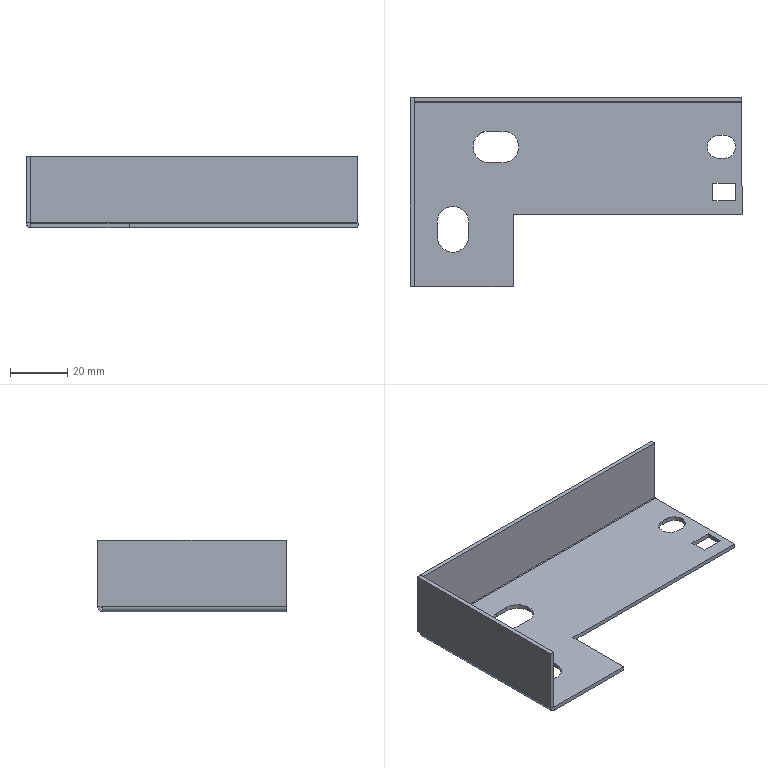Part | 1 solid | 43 faces | box 116 x 66 x 25 mm | volume 14104 mm3 | plane 31 | cylinder 12 | commonest cylinder face diameters 11 x5 8 x3 0.4 x2 3.4 x2
STEP:
#1=CARTESIAN_POINT('',(-20.,15.8,-1.5));
#2=VERTEX_POINT('',#1);
#3=CARTESIAN_POINT('',(-25.5,21.3,-1.5));
#4=VERTEX_POINT('',#3);
#5=CARTESIAN_POINT('',(-25.5,15.8,-1.5));
#6=DIRECTION('',(0.,0.,1.));
#7=DIRECTION('',(1.,0.,0.));
#8=AXIS2_PLACEMENT_3D('',#5,#6,#7);
#9=CIRCLE('',#8,5.5);
#10=EDGE_CURVE('',#2,#4,#9,.T.);
#11=ORIENTED_EDGE('',*,*,#10,.F.);
#12=CARTESIAN_POINT('',(-20.,15.8,0.));
#13=VERTEX_POINT('',#12);
#14=CARTESIAN_POINT('',(-20.,15.8,-10.));
#15=DIRECTION('',(0.,0.,1.));
#16=VECTOR('',#15,1000.);
#17=LINE('',#14,#16);
#18=EDGE_CURVE('',#2,#13,#17,.T.);
#19=ORIENTED_EDGE('',*,*,#18,.T.);
#20=CARTESIAN_POINT('',(-25.5,21.3,0.));
#21=VERTEX_POINT('',#20);
#22=CARTESIAN_POINT('',(-25.5,15.8,0.));
#23=DIRECTION('',(0.,0.,1.));
#24=DIRECTION('',(1.,0.,0.));
#25=AXIS2_PLACEMENT_3D('',#22,#23,#24);
#26=CIRCLE('',#25,5.5);
#27=EDGE_CURVE('',#13,#21,#26,.T.);
#28=ORIENTED_EDGE('',*,*,#27,.T.);
#29=CARTESIAN_POINT('',(-25.5,21.3,-10.));
#30=DIRECTION('',(0.,0.,1.));
#31=VECTOR('',#30,1000.);
#32=LINE('',#29,#31);
#33=EDGE_CURVE('',#4,#21,#32,.T.);
#34=ORIENTED_EDGE('',*,*,#33,.F.);
#35=EDGE_LOOP('',(#11,#19,#28,#34));
#36=FACE_OUTER_BOUND('',#35,.T.);
#37=CARTESIAN_POINT('',(-25.5,15.8,-10.));
#38=DIRECTION('',(0.,0.,1.));
#39=DIRECTION('',(1.,0.,0.));
#40=AXIS2_PLACEMENT_3D('',#37,#38,#39);
#41=CYLINDRICAL_SURFACE('',#40,5.5);
#42=ADVANCED_FACE('',(#36),#41,.F.);
#43=CARTESIAN_POINT('',(55.8,15.8,-1.5));
#44=VERTEX_POINT('',#43);
#45=CARTESIAN_POINT('',(51.8,19.8,-1.5));
#46=VERTEX_POINT('',#45);
#47=CARTESIAN_POINT('',(51.8,15.8,-1.5));
#48=DIRECTION('',(0.,0.,1.));
#49=DIRECTION('',(1.,0.,0.));
#50=AXIS2_PLACEMENT_3D('',#47,#48,#49);
#51=CIRCLE('',#50,4.);
#52=EDGE_CURVE('',#44,#46,#51,.T.);
#53=ORIENTED_EDGE('',*,*,#52,.F.);
#54=CARTESIAN_POINT('',(55.8,15.8,0.));
#55=VERTEX_POINT('',#54);
#56=CARTESIAN_POINT('',(55.8,15.8,-10.));
#57=DIRECTION('',(0.,0.,1.));
#58=VECTOR('',#57,1000.);
#59=LINE('',#56,#58);
#60=EDGE_CURVE('',#44,#55,#59,.T.);
#61=ORIENTED_EDGE('',*,*,#60,.T.);
#62=CARTESIAN_POINT('',(51.8,19.8,0.));
#63=VERTEX_POINT('',#62);
#64=CARTESIAN_POINT('',(51.8,15.8,0.));
#65=DIRECTION('',(0.,0.,1.));
#66=DIRECTION('',(1.,0.,0.));
#67=AXIS2_PLACEMENT_3D('',#64,#65,#66);
#68=CIRCLE('',#67,4.);
#69=EDGE_CURVE('',#55,#63,#68,.T.);
#70=ORIENTED_EDGE('',*,*,#69,.T.);
#71=CARTESIAN_POINT('',(51.8,19.8,-10.));
#72=DIRECTION('',(0.,0.,1.));
#73=VECTOR('',#72,1000.);
#74=LINE('',#71,#73);
#75=EDGE_CURVE('',#46,#63,#74,.T.);
#76=ORIENTED_EDGE('',*,*,#75,.F.);
#77=EDGE_LOOP('',(#53,#61,#70,#76));
#78=FACE_OUTER_BOUND('',#77,.T.);
#79=CARTESIAN_POINT('',(51.8,15.8,-10.));
#80=DIRECTION('',(0.,0.,1.));
#81=DIRECTION('',(1.,0.,0.));
#82=AXIS2_PLACEMENT_3D('',#79,#80,#81);
#83=CYLINDRICAL_SURFACE('',#82,4.);
#84=ADVANCED_FACE('',(#78),#83,.F.);
#85=CARTESIAN_POINT('',(-30.5,21.3,-1.5));
#86=VERTEX_POINT('',#85);
#87=CARTESIAN_POINT('',(0.,21.3,-1.5));
#88=DIRECTION('',(-1.,0.,0.));
#89=VECTOR('',#88,1000.);
#90=LINE('',#87,#89);
#91=EDGE_CURVE('',#4,#86,#90,.T.);
#92=ORIENTED_EDGE('',*,*,#91,.T.);
#93=CARTESIAN_POINT('',(-30.5,10.3,-1.5));
#94=VERTEX_POINT('',#93);
#95=CARTESIAN_POINT('',(-30.5,15.8,-1.5));
#96=DIRECTION('',(0.,0.,1.));
#97=DIRECTION('',(1.,0.,0.));
#98=AXIS2_PLACEMENT_3D('',#95,#96,#97);
#99=CIRCLE('',#98,5.5);
#100=EDGE_CURVE('',#86,#94,#99,.T.);
#101=ORIENTED_EDGE('',*,*,#100,.T.);
#102=CARTESIAN_POINT('',(-25.5,10.3,-1.5));
#103=VERTEX_POINT('',#102);
#104=CARTESIAN_POINT('',(0.,10.3,-1.5));
#105=DIRECTION('',(1.,0.,0.));
#106=VECTOR('',#105,1000.);
#107=LINE('',#104,#106);
#108=EDGE_CURVE('',#94,#103,#107,.T.);
#109=ORIENTED_EDGE('',*,*,#108,.T.);
#110=CARTESIAN_POINT('',(-25.5,15.8,-1.5));
#111=DIRECTION('',(0.,0.,1.));
#112=DIRECTION('',(1.,0.,0.));
#113=AXIS2_PLACEMENT_3D('',#110,#111,#112);
#114=CIRCLE('',#113,5.5);
#115=EDGE_CURVE('',#103,#2,#114,.T.);
#116=ORIENTED_EDGE('',*,*,#115,.T.);
#117=ORIENTED_EDGE('',*,*,#10,.T.);
#118=EDGE_LOOP('',(#92,#101,#109,#116,#117));
#119=FACE_BOUND('',#118,.T.);
#120=CARTESIAN_POINT('',(58.,-8.,-1.5));
#121=VERTEX_POINT('',#120);
#122=CARTESIAN_POINT('',(58.,31.3,-1.5));
#123=VERTEX_POINT('',#122);
#124=CARTESIAN_POINT('',(58.,33.,-1.5));
#125=DIRECTION('',(0.,1.,0.));
#126=VECTOR('',#125,1000.);
#127=LINE('',#124,#126);
#128=EDGE_CURVE('',#121,#123,#127,.T.);
#129=ORIENTED_EDGE('',*,*,#128,.F.);
#130=CARTESIAN_POINT('',(-22.,-8.,-1.5));
#131=VERTEX_POINT('',#130);
#132=CARTESIAN_POINT('',(0.,-8.,-1.5));
#133=DIRECTION('',(-1.,0.,0.));
#134=VECTOR('',#133,1000.);
#135=LINE('',#132,#134);
#136=EDGE_CURVE('',#121,#131,#135,.T.);
#137=ORIENTED_EDGE('',*,*,#136,.T.);
#138=CARTESIAN_POINT('',(-22.,-33.,-1.5));
#139=VERTEX_POINT('',#138);
#140=CARTESIAN_POINT('',(-22.,0.,-1.5));
#141=DIRECTION('',(0.,-1.,0.));
#142=VECTOR('',#141,1000.);
#143=LINE('',#140,#142);
#144=EDGE_CURVE('',#131,#139,#143,.T.);
#145=ORIENTED_EDGE('',*,*,#144,.T.);
#146=CARTESIAN_POINT('',(-56.3,-33.,-1.5));
#147=VERTEX_POINT('',#146);
#148=CARTESIAN_POINT('',(-58.,-33.,-1.5));
#149=DIRECTION('',(1.,0.,0.));
#150=VECTOR('',#149,1000.);
#151=LINE('',#148,#150);
#152=EDGE_CURVE('',#147,#139,#151,.T.);
#153=ORIENTED_EDGE('',*,*,#152,.F.);
#154=CARTESIAN_POINT('',(-56.3,31.3,-1.5));
#155=VERTEX_POINT('',#154);
#156=CARTESIAN_POINT('',(-56.3,-33.,-1.5));
#157=DIRECTION('',(0.,1.,0.));
#158=VECTOR('',#157,1000.);
#159=LINE('',#156,#158);
#160=EDGE_CURVE('',#147,#155,#159,.T.);
#161=ORIENTED_EDGE('',*,*,#160,.T.);
#162=CARTESIAN_POINT('',(-56.3,31.3,-1.5));
#163=DIRECTION('',(1.,0.,0.));
#164=VECTOR('',#163,1000.);
#165=LINE('',#162,#164);
#166=EDGE_CURVE('',#155,#123,#165,.T.);
#167=ORIENTED_EDGE('',*,*,#166,.T.);
#168=EDGE_LOOP('',(#129,#137,#145,#153,#161,#167));
#169=FACE_OUTER_BOUND('',#168,.T.);
#170=CARTESIAN_POINT('',(-37.5,-15.5,-1.5));
#171=VERTEX_POINT('',#170);
#172=CARTESIAN_POINT('',(-37.5,-10.5,-1.5));
#173=VERTEX_POINT('',#172);
#174=CARTESIAN_POINT('',(-37.5,0.,-1.5));
#175=DIRECTION('',(0.,1.,0.));
#176=VECTOR('',#175,1000.);
#177=LINE('',#174,#176);
#178=EDGE_CURVE('',#171,#173,#177,.T.);
#179=ORIENTED_EDGE('',*,*,#178,.T.);
#180=CARTESIAN_POINT('',(-48.5,-10.5,-1.5));
#181=VERTEX_POINT('',#180);
#182=CARTESIAN_POINT('',(-43.,-10.5,-1.5));
#183=DIRECTION('',(0.,0.,1.));
#184=DIRECTION('',(1.,0.,0.));
#185=AXIS2_PLACEMENT_3D('',#182,#183,#184);
#186=CIRCLE('',#185,5.5);
#187=EDGE_CURVE('',#173,#181,#186,.T.);
#188=ORIENTED_EDGE('',*,*,#187,.T.);
#189=CARTESIAN_POINT('',(-48.5,-15.5,-1.5));
#190=VERTEX_POINT('',#189);
#191=CARTESIAN_POINT('',(-48.5,0.,-1.5));
#192=DIRECTION('',(0.,-1.,0.));
#193=VECTOR('',#192,1000.);
#194=LINE('',#191,#193);
#195=EDGE_CURVE('',#181,#190,#194,.T.);
#196=ORIENTED_EDGE('',*,*,#195,.T.);
#197=CARTESIAN_POINT('',(-43.,-15.5,-1.5));
#198=DIRECTION('',(0.,0.,1.));
#199=DIRECTION('',(1.,0.,0.));
#200=AXIS2_PLACEMENT_3D('',#197,#198,#199);
#201=CIRCLE('',#200,5.5);
#202=EDGE_CURVE('',#190,#171,#201,.T.);
#203=ORIENTED_EDGE('',*,*,#202,.T.);
#204=EDGE_LOOP('',(#179,#188,#196,#203));
#205=FACE_BOUND('',#204,.T.);
#206=CARTESIAN_POINT('',(49.8,19.8,-1.5));
#207=VERTEX_POINT('',#206);
#208=CARTESIAN_POINT('',(0.,19.8,-1.5));
#209=DIRECTION('',(-1.,0.,0.));
#210=VECTOR('',#209,1000.);
#211=LINE('',#208,#210);
#212=EDGE_CURVE('',#46,#207,#211,.T.);
#213=ORIENTED_EDGE('',*,*,#212,.T.);
#214=CARTESIAN_POINT('',(49.8,11.8,-1.5));
#215=VERTEX_POINT('',#214);
#216=CARTESIAN_POINT('',(49.8,15.8,-1.5));
#217=DIRECTION('',(0.,0.,1.));
#218=DIRECTION('',(1.,0.,0.));
#219=AXIS2_PLACEMENT_3D('',#216,#217,#218);
#220=CIRCLE('',#219,4.);
#221=EDGE_CURVE('',#207,#215,#220,.T.);
#222=ORIENTED_EDGE('',*,*,#221,.T.);
#223=CARTESIAN_POINT('',(51.8,11.8,-1.5));
#224=VERTEX_POINT('',#223);
#225=CARTESIAN_POINT('',(0.,11.8,-1.5));
#226=DIRECTION('',(1.,0.,0.));
#227=VECTOR('',#226,1000.);
#228=LINE('',#225,#227);
#229=EDGE_CURVE('',#215,#224,#228,.T.);
#230=ORIENTED_EDGE('',*,*,#229,.T.);
#231=CARTESIAN_POINT('',(51.8,15.8,-1.5));
#232=DIRECTION('',(0.,0.,1.));
#233=DIRECTION('',(1.,0.,0.));
#234=AXIS2_PLACEMENT_3D('',#231,#232,#233);
#235=CIRCLE('',#234,4.);
#236=EDGE_CURVE('',#224,#44,#235,.T.);
#237=ORIENTED_EDGE('',*,*,#236,.T.);
#238=ORIENTED_EDGE('',*,*,#52,.T.);
#239=EDGE_LOOP('',(#213,#222,#230,#237,#238));
#240=FACE_BOUND('',#239,.T.);
#241=CARTESIAN_POINT('',(55.8,3.,-1.5));
#242=VERTEX_POINT('',#241);
#243=CARTESIAN_POINT('',(55.8,-3.,-1.5));
#244=VERTEX_POINT('',#243);
#245=CARTESIAN_POINT('',(55.8,0.,-1.5));
#246=DIRECTION('',(0.,-1.,0.));
#247=VECTOR('',#246,1000.);
#248=LINE('',#245,#247);
#249=EDGE_CURVE('',#242,#244,#248,.T.);
#250=ORIENTED_EDGE('',*,*,#249,.F.);
#251=CARTESIAN_POINT('',(47.8,3.,-1.5));
#252=VERTEX_POINT('',#251);
#253=CARTESIAN_POINT('',(0.,3.,-1.5));
#254=DIRECTION('',(1.,0.,0.));
#255=VECTOR('',#254,1000.);
#256=LINE('',#253,#255);
#257=EDGE_CURVE('',#252,#242,#256,.T.);
#258=ORIENTED_EDGE('',*,*,#257,.F.);
#259=CARTESIAN_POINT('',(47.8,-3.,-1.5));
#260=VERTEX_POINT('',#259);
#261=CARTESIAN_POINT('',(47.8,0.,-1.5));
#262=DIRECTION('',(0.,1.,0.));
#263=VECTOR('',#262,1000.);
#264=LINE('',#261,#263);
#265=EDGE_CURVE('',#260,#252,#264,.T.);
#266=ORIENTED_EDGE('',*,*,#265,.F.);
#267=CARTESIAN_POINT('',(0.,-3.,-1.5));
#268=DIRECTION('',(-1.,0.,0.));
#269=VECTOR('',#268,1000.);
#270=LINE('',#267,#269);
#271=EDGE_CURVE('',#244,#260,#270,.T.);
#272=ORIENTED_EDGE('',*,*,#271,.F.);
#273=EDGE_LOOP('',(#250,#258,#266,#272));
#274=FACE_BOUND('',#273,.T.);
#275=CARTESIAN_POINT('',(0.,0.,-1.5));
#276=DIRECTION('',(0.,0.,1.));
#277=DIRECTION('',(1.,0.,0.));
#278=AXIS2_PLACEMENT_3D('',#275,#276,#277);
#279=PLANE('',#278);
#280=ADVANCED_FACE('',(#119,#169,#205,#240,#274),#279,.F.);
#281=CARTESIAN_POINT('',(-30.5,21.3,0.));
#282=VERTEX_POINT('',#281);
#283=CARTESIAN_POINT('',(-30.5,10.3,0.));
#284=VERTEX_POINT('',#283);
#285=CARTESIAN_POINT('',(-30.5,15.8,0.));
#286=DIRECTION('',(0.,0.,1.));
#287=DIRECTION('',(1.,0.,0.));
#288=AXIS2_PLACEMENT_3D('',#285,#286,#287);
#289=CIRCLE('',#288,5.5);
#290=EDGE_CURVE('',#282,#284,#289,.T.);
#291=ORIENTED_EDGE('',*,*,#290,.F.);
#292=CARTESIAN_POINT('',(-30.5,21.3,0.));
#293=DIRECTION('',(-1.,0.,0.));
#294=VECTOR('',#293,1000.);
#295=LINE('',#292,#294);
#296=EDGE_CURVE('',#21,#282,#295,.T.);
#297=ORIENTED_EDGE('',*,*,#296,.F.);
#298=ORIENTED_EDGE('',*,*,#27,.F.);
#299=CARTESIAN_POINT('',(-25.5,10.3,0.));
#300=VERTEX_POINT('',#299);
#301=CARTESIAN_POINT('',(-25.5,15.8,0.));
#302=DIRECTION('',(0.,0.,1.));
#303=DIRECTION('',(1.,0.,0.));
#304=AXIS2_PLACEMENT_3D('',#301,#302,#303);
#305=CIRCLE('',#304,5.5);
#306=EDGE_CURVE('',#300,#13,#305,.T.);
#307=ORIENTED_EDGE('',*,*,#306,.F.);
#308=CARTESIAN_POINT('',(-30.5,10.3,0.));
#309=DIRECTION('',(1.,0.,0.));
#310=VECTOR('',#309,1000.);
#311=LINE('',#308,#310);
#312=EDGE_CURVE('',#284,#300,#311,.T.);
#313=ORIENTED_EDGE('',*,*,#312,.F.);
#314=EDGE_LOOP('',(#291,#297,#298,#307,#313));
#315=FACE_BOUND('',#314,.T.);
#316=CARTESIAN_POINT('',(58.,-8.,0.));
#317=VERTEX_POINT('',#316);
#318=CARTESIAN_POINT('',(-22.,-8.,0.));
#319=VERTEX_POINT('',#318);
#320=CARTESIAN_POINT('',(0.,-8.,0.));
#321=DIRECTION('',(-1.,0.,0.));
#322=VECTOR('',#321,1000.);
#323=LINE('',#320,#322);
#324=EDGE_CURVE('',#317,#319,#323,.T.);
#325=ORIENTED_EDGE('',*,*,#324,.F.);
#326=CARTESIAN_POINT('',(58.,31.3,0.));
#327=VERTEX_POINT('',#326);
#328=CARTESIAN_POINT('',(58.,33.,0.));
#329=DIRECTION('',(0.,1.,0.));
#330=VECTOR('',#329,1000.);
#331=LINE('',#328,#330);
#332=EDGE_CURVE('',#317,#327,#331,.T.);
#333=ORIENTED_EDGE('',*,*,#332,.T.);
#334=CARTESIAN_POINT('',(-56.3,31.3,0.));
#335=VERTEX_POINT('',#334);
#336=CARTESIAN_POINT('',(-56.3,31.3,0.));
#337=DIRECTION('',(1.,0.,0.));
#338=VECTOR('',#337,1000.);
#339=LINE('',#336,#338);
#340=EDGE_CURVE('',#335,#327,#339,.T.);
#341=ORIENTED_EDGE('',*,*,#340,.F.);
#342=CARTESIAN_POINT('',(-56.3,-33.,0.));
#343=VERTEX_POINT('',#342);
#344=CARTESIAN_POINT('',(-56.3,-33.,0.));
#345=DIRECTION('',(0.,1.,0.));
#346=VECTOR('',#345,1000.);
#347=LINE('',#344,#346);
#348=EDGE_CURVE('',#343,#335,#347,.T.);
#349=ORIENTED_EDGE('',*,*,#348,.F.);
#350=CARTESIAN_POINT('',(-22.,-33.,0.));
#351=VERTEX_POINT('',#350);
#352=CARTESIAN_POINT('',(-58.,-33.,0.));
#353=DIRECTION('',(1.,0.,0.));
#354=VECTOR('',#353,1000.);
#355=LINE('',#352,#354);
#356=EDGE_CURVE('',#343,#351,#355,.T.);
#357=ORIENTED_EDGE('',*,*,#356,.T.);
#358=CARTESIAN_POINT('',(-22.,0.,0.));
#359=DIRECTION('',(0.,-1.,0.));
#360=VECTOR('',#359,1000.);
#361=LINE('',#358,#360);
#362=EDGE_CURVE('',#319,#351,#361,.T.);
#363=ORIENTED_EDGE('',*,*,#362,.F.);
#364=EDGE_LOOP('',(#325,#333,#341,#349,#357,#363));
#365=FACE_OUTER_BOUND('',#364,.T.);
#366=CARTESIAN_POINT('',(49.8,19.8,0.));
#367=VERTEX_POINT('',#366);
#368=CARTESIAN_POINT('',(49.8,11.8,0.));
#369=VERTEX_POINT('',#368);
#370=CARTESIAN_POINT('',(49.8,15.8,0.));
#371=DIRECTION('',(0.,0.,1.));
#372=DIRECTION('',(1.,0.,0.));
#373=AXIS2_PLACEMENT_3D('',#370,#371,#372);
#374=CIRCLE('',#373,4.);
#375=EDGE_CURVE('',#367,#369,#374,.T.);
#376=ORIENTED_EDGE('',*,*,#375,.F.);
#377=CARTESIAN_POINT('',(49.8,19.8,0.));
#378=DIRECTION('',(-1.,0.,0.));
#379=VECTOR('',#378,1000.);
#380=LINE('',#377,#379);
#381=EDGE_CURVE('',#63,#367,#380,.T.);
#382=ORIENTED_EDGE('',*,*,#381,.F.);
#383=ORIENTED_EDGE('',*,*,#69,.F.);
#384=CARTESIAN_POINT('',(51.8,11.8,0.));
#385=VERTEX_POINT('',#384);
#386=CARTESIAN_POINT('',(51.8,15.8,0.));
#387=DIRECTION('',(0.,0.,1.));
#388=DIRECTION('',(1.,0.,0.));
#389=AXIS2_PLACEMENT_3D('',#386,#387,#388);
#390=CIRCLE('',#389,4.);
#391=EDGE_CURVE('',#385,#55,#390,.T.);
#392=ORIENTED_EDGE('',*,*,#391,.F.);
#393=CARTESIAN_POINT('',(49.8,11.8,0.));
#394=DIRECTION('',(1.,0.,0.));
#395=VECTOR('',#394,1000.);
#396=LINE('',#393,#395);
#397=EDGE_CURVE('',#369,#385,#396,.T.);
#398=ORIENTED_EDGE('',*,*,#397,.F.);
#399=EDGE_LOOP('',(#376,#382,#383,#392,#398));
#400=FACE_BOUND('',#399,.T.);
#401=CARTESIAN_POINT('',(-37.5,-10.5,0.));
#402=VERTEX_POINT('',#401);
#403=CARTESIAN_POINT('',(-48.5,-10.5,0.));
#404=VERTEX_POINT('',#403);
#405=CARTESIAN_POINT('',(-43.,-10.5,0.));
#406=DIRECTION('',(0.,0.,1.));
#407=DIRECTION('',(1.,0.,0.));
#408=AXIS2_PLACEMENT_3D('',#405,#406,#407);
#409=CIRCLE('',#408,5.5);
#410=EDGE_CURVE('',#402,#404,#409,.T.);
#411=ORIENTED_EDGE('',*,*,#410,.F.);
#412=CARTESIAN_POINT('',(-37.5,-15.5,0.));
#413=VERTEX_POINT('',#412);
#414=CARTESIAN_POINT('',(-37.5,-10.5,0.));
#415=DIRECTION('',(0.,1.,0.));
#416=VECTOR('',#415,1000.);
#417=LINE('',#414,#416);
#418=EDGE_CURVE('',#413,#402,#417,.T.);
#419=ORIENTED_EDGE('',*,*,#418,.F.);
#420=CARTESIAN_POINT('',(-48.5,-15.5,0.));
#421=VERTEX_POINT('',#420);
#422=CARTESIAN_POINT('',(-43.,-15.5,0.));
#423=DIRECTION('',(0.,0.,1.));
#424=DIRECTION('',(1.,0.,0.));
#425=AXIS2_PLACEMENT_3D('',#422,#423,#424);
#426=CIRCLE('',#425,5.5);
#427=EDGE_CURVE('',#421,#413,#426,.T.);
#428=ORIENTED_EDGE('',*,*,#427,.F.);
#429=CARTESIAN_POINT('',(-48.5,-10.5,0.));
#430=DIRECTION('',(0.,-1.,0.));
#431=VECTOR('',#430,1000.);
#432=LINE('',#429,#431);
#433=EDGE_CURVE('',#404,#421,#432,.T.);
#434=ORIENTED_EDGE('',*,*,#433,.F.);
#435=EDGE_LOOP('',(#411,#419,#428,#434));
#436=FACE_BOUND('',#435,.T.);
#437=CARTESIAN_POINT('',(47.8,3.,0.));
#438=VERTEX_POINT('',#437);
#439=CARTESIAN_POINT('',(55.8,3.,0.));
#440=VERTEX_POINT('',#439);
#441=CARTESIAN_POINT('',(0.,3.,0.));
#442=DIRECTION('',(1.,0.,0.));
#443=VECTOR('',#442,1000.);
#444=LINE('',#441,#443);
#445=EDGE_CURVE('',#438,#440,#444,.T.);
#446=ORIENTED_EDGE('',*,*,#445,.T.);
#447=CARTESIAN_POINT('',(55.8,-3.,0.));
#448=VERTEX_POINT('',#447);
#449=CARTESIAN_POINT('',(55.8,0.,0.));
#450=DIRECTION('',(0.,-1.,0.));
#451=VECTOR('',#450,1000.);
#452=LINE('',#449,#451);
#453=EDGE_CURVE('',#440,#448,#452,.T.);
#454=ORIENTED_EDGE('',*,*,#453,.T.);
#455=CARTESIAN_POINT('',(47.8,-3.,0.));
#456=VERTEX_POINT('',#455);
#457=CARTESIAN_POINT('',(0.,-3.,0.));
#458=DIRECTION('',(-1.,0.,0.));
#459=VECTOR('',#458,1000.);
#460=LINE('',#457,#459);
#461=EDGE_CURVE('',#448,#456,#460,.T.);
#462=ORIENTED_EDGE('',*,*,#461,.T.);
#463=CARTESIAN_POINT('',(47.8,0.,0.));
#464=DIRECTION('',(0.,1.,0.));
#465=VECTOR('',#464,1000.);
#466=LINE('',#463,#465);
#467=EDGE_CURVE('',#456,#438,#466,.T.);
#468=ORIENTED_EDGE('',*,*,#467,.T.);
#469=EDGE_LOOP('',(#446,#454,#462,#468));
#470=FACE_BOUND('',#469,.T.);
#471=CARTESIAN_POINT('',(0.,0.,0.));
#472=DIRECTION('',(0.,0.,1.));
#473=DIRECTION('',(1.,0.,0.));
#474=AXIS2_PLACEMENT_3D('',#471,#472,#473);
#475=PLANE('',#474);
#476=ADVANCED_FACE('',(#315,#365,#400,#436,#470),#475,.T.);
#477=CARTESIAN_POINT('',(-58.,31.3,0.2));
#478=VERTEX_POINT('',#477);
#479=CARTESIAN_POINT('',(-56.5,31.3,0.2));
#480=VERTEX_POINT('',#479);
#481=CARTESIAN_POINT('',(-58.,31.3,0.2));
#482=DIRECTION('',(1.,0.,0.));
#483=VECTOR('',#482,1000.);
#484=LINE('',#481,#483);
#485=EDGE_CURVE('',#478,#480,#484,.T.);
#486=ORIENTED_EDGE('',*,*,#485,.F.);
#487=CARTESIAN_POINT('',(-58.,33.,0.2));
#488=VERTEX_POINT('',#487);
#489=CARTESIAN_POINT('',(-58.,33.,0.2));
#490=DIRECTION('',(0.,1.,0.));
#491=VECTOR('',#490,1000.);
#492=LINE('',#489,#491);
#493=EDGE_CURVE('',#478,#488,#492,.T.);
#494=ORIENTED_EDGE('',*,*,#493,.T.);
#495=CARTESIAN_POINT('',(-56.5,33.,0.2));
#496=VERTEX_POINT('',#495);
#497=CARTESIAN_POINT('',(-58.,33.,0.2));
#498=DIRECTION('',(-1.,0.,0.));
#499=VECTOR('',#498,1000.);
#500=LINE('',#497,#499);
#501=EDGE_CURVE('',#496,#488,#500,.T.);
#502=ORIENTED_EDGE('',*,*,#501,.F.);
#503=CARTESIAN_POINT('',(-56.5,33.,0.2));
#504=DIRECTION('',(0.,-1.,0.));
#505=VECTOR('',#504,1000.);
#506=LINE('',#503,#505);
#507=EDGE_CURVE('',#496,#480,#506,.T.);
#508=ORIENTED_EDGE('',*,*,#507,.T.);
#509=EDGE_LOOP('',(#486,#494,#502,#508));
#510=FACE_OUTER_BOUND('',#509,.T.);
#511=CARTESIAN_POINT('',(0.,0.,0.2));
#512=DIRECTION('',(0.,0.,-1.));
#513=DIRECTION('',(-1.,0.,0.));
#514=AXIS2_PLACEMENT_3D('',#511,#512,#513);
#515=PLANE('',#514);
#516=ADVANCED_FACE('',(#510),#515,.T.);
#517=CARTESIAN_POINT('',(-58.,-33.,0.2));
#518=VERTEX_POINT('',#517);
#519=CARTESIAN_POINT('',(-58.,33.,0.2));
#520=DIRECTION('',(0.,1.,0.));
#521=VECTOR('',#520,1000.);
#522=LINE('',#519,#521);
#523=EDGE_CURVE('',#518,#478,#522,.T.);
#524=ORIENTED_EDGE('',*,*,#523,.T.);
#525=CARTESIAN_POINT('',(-56.3,31.3,0.2));
#526=DIRECTION('',(0.,-1.,0.));
#527=DIRECTION('',(0.,0.,1.));
#528=AXIS2_PLACEMENT_3D('',#525,#526,#527);
#529=CIRCLE('',#528,1.7);
#530=EDGE_CURVE('',#478,#155,#529,.T.);
#531=ORIENTED_EDGE('',*,*,#530,.T.);
#532=ORIENTED_EDGE('',*,*,#160,.F.);
#533=CARTESIAN_POINT('',(-56.3,-33.,0.2));
#534=DIRECTION('',(0.,-1.,0.));
#535=DIRECTION('',(0.,0.,-1.));
#536=AXIS2_PLACEMENT_3D('',#533,#534,#535);
#537=CIRCLE('',#536,1.7);
#538=EDGE_CURVE('',#518,#147,#537,.T.);
#539=ORIENTED_EDGE('',*,*,#538,.F.);
#540=EDGE_LOOP('',(#524,#531,#532,#539));
#541=FACE_OUTER_BOUND('',#540,.T.);
#542=CARTESIAN_POINT('',(-56.3,-33.,0.2));
#543=DIRECTION('',(0.,-1.,0.));
#544=DIRECTION('',(-1.,0.,0.));
#545=AXIS2_PLACEMENT_3D('',#542,#543,#544);
#546=CYLINDRICAL_SURFACE('',#545,1.7);
#547=ADVANCED_FACE('',(#541),#546,.T.);
#548=CARTESIAN_POINT('',(-22.,-33.,23.5));
#549=DIRECTION('',(0.,0.,-1.));
#550=VECTOR('',#549,1000.);
#551=LINE('',#548,#550);
#552=EDGE_CURVE('',#351,#139,#551,.T.);
#553=ORIENTED_EDGE('',*,*,#552,.F.);
#554=ORIENTED_EDGE('',*,*,#356,.F.);
#555=CARTESIAN_POINT('',(-56.3,-33.,0.));
#556=DIRECTION('',(0.,0.,-1.));
#557=VECTOR('',#556,1000.);
#558=LINE('',#555,#557);
#559=EDGE_CURVE('',#343,#147,#558,.T.);
#560=ORIENTED_EDGE('',*,*,#559,.T.);
#561=ORIENTED_EDGE('',*,*,#152,.T.);
#562=EDGE_LOOP('',(#553,#554,#560,#561));
#563=FACE_OUTER_BOUND('',#562,.T.);
#564=CARTESIAN_POINT('',(-58.,-33.,-1.5));
#565=DIRECTION('',(0.,-1.,0.));
#566=DIRECTION('',(0.,0.,-1.));
#567=AXIS2_PLACEMENT_3D('',#564,#565,#566);
#568=PLANE('',#567);
#569=ADVANCED_FACE('',(#563),#568,.T.);
#570=CARTESIAN_POINT('',(58.,-8.,-1.5));
#571=DIRECTION('',(0.,0.,1.));
#572=VECTOR('',#571,1000.);
#573=LINE('',#570,#572);
#574=EDGE_CURVE('',#121,#317,#573,.T.);
#575=ORIENTED_EDGE('',*,*,#574,.F.);
#576=ORIENTED_EDGE('',*,*,#128,.T.);
#577=CARTESIAN_POINT('',(58.,31.3,0.));
#578=DIRECTION('',(0.,0.,-1.));
#579=VECTOR('',#578,1000.);
#580=LINE('',#577,#579);
#581=EDGE_CURVE('',#327,#123,#580,.T.);
#582=ORIENTED_EDGE('',*,*,#581,.F.);
#583=ORIENTED_EDGE('',*,*,#332,.F.);
#584=EDGE_LOOP('',(#575,#576,#582,#583));
#585=FACE_OUTER_BOUND('',#584,.T.);
#586=CARTESIAN_POINT('',(58.,33.,-1.5));
#587=DIRECTION('',(1.,0.,0.));
#588=DIRECTION('',(0.,1.,0.));
#589=AXIS2_PLACEMENT_3D('',#586,#587,#588);
#590=PLANE('',#589);
#591=ADVANCED_FACE('',(#585),#590,.T.);
#592=CARTESIAN_POINT('',(-37.5,-10.5,-10.));
#593=DIRECTION('',(0.,0.,1.));
#594=VECTOR('',#593,1000.);
#595=LINE('',#592,#594);
#596=EDGE_CURVE('',#173,#402,#595,.T.);
#597=ORIENTED_EDGE('',*,*,#596,.T.);
#598=ORIENTED_EDGE('',*,*,#410,.T.);
#599=CARTESIAN_POINT('',(-48.5,-10.5,-10.));
#600=DIRECTION('',(0.,0.,1.));
#601=VECTOR('',#600,1000.);
#602=LINE('',#599,#601);
#603=EDGE_CURVE('',#181,#404,#602,.T.);
#604=ORIENTED_EDGE('',*,*,#603,.F.);
#605=ORIENTED_EDGE('',*,*,#187,.F.);
#606=EDGE_LOOP('',(#597,#598,#604,#605));
#607=FACE_OUTER_BOUND('',#606,.T.);
#608=CARTESIAN_POINT('',(-43.,-10.5,-10.));
#609=DIRECTION('',(0.,0.,1.));
#610=DIRECTION('',(1.,0.,0.));
#611=AXIS2_PLACEMENT_3D('',#608,#609,#610);
#612=CYLINDRICAL_SURFACE('',#611,5.5);
#613=ADVANCED_FACE('',(#607),#612,.F.);
#614=CARTESIAN_POINT('',(-37.5,-15.5,-10.));
#615=DIRECTION('',(0.,0.,1.));
#616=VECTOR('',#615,1000.);
#617=LINE('',#614,#616);
#618=EDGE_CURVE('',#171,#413,#617,.T.);
#619=ORIENTED_EDGE('',*,*,#618,.T.);
#620=ORIENTED_EDGE('',*,*,#418,.T.);
#621=ORIENTED_EDGE('',*,*,#596,.F.);
#622=ORIENTED_EDGE('',*,*,#178,.F.);
#623=EDGE_LOOP('',(#619,#620,#621,#622));
#624=FACE_OUTER_BOUND('',#623,.T.);
#625=CARTESIAN_POINT('',(-37.5,-10.5,-10.));
#626=DIRECTION('',(1.,0.,0.));
#627=DIRECTION('',(0.,0.,-1.));
#628=AXIS2_PLACEMENT_3D('',#625,#626,#627);
#629=PLANE('',#628);
#630=ADVANCED_FACE('',(#624),#629,.F.);
#631=CARTESIAN_POINT('',(-48.5,-15.5,-10.));
#632=DIRECTION('',(0.,0.,1.));
#633=VECTOR('',#632,1000.);
#634=LINE('',#631,#633);
#635=EDGE_CURVE('',#190,#421,#634,.T.);
#636=ORIENTED_EDGE('',*,*,#635,.T.);
#637=ORIENTED_EDGE('',*,*,#427,.T.);
#638=ORIENTED_EDGE('',*,*,#618,.F.);
#639=ORIENTED_EDGE('',*,*,#202,.F.);
#640=EDGE_LOOP('',(#636,#637,#638,#639));
#641=FACE_OUTER_BOUND('',#640,.T.);
#642=CARTESIAN_POINT('',(-43.,-15.5,-10.));
#643=DIRECTION('',(0.,0.,1.));
#644=DIRECTION('',(1.,0.,0.));
#645=AXIS2_PLACEMENT_3D('',#642,#643,#644);
#646=CYLINDRICAL_SURFACE('',#645,5.5);
#647=ADVANCED_FACE('',(#641),#646,.F.);
#648=ORIENTED_EDGE('',*,*,#603,.T.);
#649=ORIENTED_EDGE('',*,*,#433,.T.);
#650=ORIENTED_EDGE('',*,*,#635,.F.);
#651=ORIENTED_EDGE('',*,*,#195,.F.);
#652=EDGE_LOOP('',(#648,#649,#650,#651));
#653=FACE_OUTER_BOUND('',#652,.T.);
#654=CARTESIAN_POINT('',(-48.5,-10.5,-10.));
#655=DIRECTION('',(-1.,0.,0.));
#656=DIRECTION('',(0.,0.,1.));
#657=AXIS2_PLACEMENT_3D('',#654,#655,#656);
#658=PLANE('',#657);
#659=ADVANCED_FACE('',(#653),#658,.F.);
#660=CARTESIAN_POINT('',(49.8,19.8,-10.));
#661=DIRECTION('',(0.,0.,1.));
#662=VECTOR('',#661,1000.);
#663=LINE('',#660,#662);
#664=EDGE_CURVE('',#207,#367,#663,.T.);
#665=ORIENTED_EDGE('',*,*,#664,.T.);
#666=ORIENTED_EDGE('',*,*,#375,.T.);
#667=CARTESIAN_POINT('',(49.8,11.8,-10.));
#668=DIRECTION('',(0.,0.,1.));
#669=VECTOR('',#668,1000.);
#670=LINE('',#667,#669);
#671=EDGE_CURVE('',#215,#369,#670,.T.);
#672=ORIENTED_EDGE('',*,*,#671,.F.);
#673=ORIENTED_EDGE('',*,*,#221,.F.);
#674=EDGE_LOOP('',(#665,#666,#672,#673));
#675=FACE_OUTER_BOUND('',#674,.T.);
#676=CARTESIAN_POINT('',(49.8,15.8,-10.));
#677=DIRECTION('',(0.,0.,1.));
#678=DIRECTION('',(1.,0.,0.));
#679=AXIS2_PLACEMENT_3D('',#676,#677,#678);
#680=CYLINDRICAL_SURFACE('',#679,4.);
#681=ADVANCED_FACE('',(#675),#680,.F.);
#682=ORIENTED_EDGE('',*,*,#75,.T.);
#683=ORIENTED_EDGE('',*,*,#381,.T.);
#684=ORIENTED_EDGE('',*,*,#664,.F.);
#685=ORIENTED_EDGE('',*,*,#212,.F.);
#686=EDGE_LOOP('',(#682,#683,#684,#685));
#687=FACE_OUTER_BOUND('',#686,.T.);
#688=CARTESIAN_POINT('',(49.8,19.8,-10.));
#689=DIRECTION('',(0.,1.,0.));
#690=DIRECTION('',(0.,0.,1.));
#691=AXIS2_PLACEMENT_3D('',#688,#689,#690);
#692=PLANE('',#691);
#693=ADVANCED_FACE('',(#687),#692,.F.);
#694=ORIENTED_EDGE('',*,*,#60,.F.);
#695=ORIENTED_EDGE('',*,*,#236,.F.);
#696=CARTESIAN_POINT('',(51.8,11.8,-10.));
#697=DIRECTION('',(0.,0.,1.));
#698=VECTOR('',#697,1000.);
#699=LINE('',#696,#698);
#700=EDGE_CURVE('',#224,#385,#699,.T.);
#701=ORIENTED_EDGE('',*,*,#700,.T.);
#702=ORIENTED_EDGE('',*,*,#391,.T.);
#703=EDGE_LOOP('',(#694,#695,#701,#702));
#704=FACE_OUTER_BOUND('',#703,.T.);
#705=CARTESIAN_POINT('',(51.8,15.8,-10.));
#706=DIRECTION('',(0.,0.,1.));
#707=DIRECTION('',(1.,0.,0.));
#708=AXIS2_PLACEMENT_3D('',#705,#706,#707);
#709=CYLINDRICAL_SURFACE('',#708,4.);
#710=ADVANCED_FACE('',(#704),#709,.F.);
#711=ORIENTED_EDGE('',*,*,#671,.T.);
#712=ORIENTED_EDGE('',*,*,#397,.T.);
#713=ORIENTED_EDGE('',*,*,#700,.F.);
#714=ORIENTED_EDGE('',*,*,#229,.F.);
#715=EDGE_LOOP('',(#711,#712,#713,#714));
#716=FACE_OUTER_BOUND('',#715,.T.);
#717=CARTESIAN_POINT('',(49.8,11.8,-10.));
#718=DIRECTION('',(0.,-1.,0.));
#719=DIRECTION('',(0.,0.,-1.));
#720=AXIS2_PLACEMENT_3D('',#717,#718,#719);
#721=PLANE('',#720);
#722=ADVANCED_FACE('',(#716),#721,.F.);
#723=CARTESIAN_POINT('',(-56.5,-33.,0.2));
#724=VERTEX_POINT('',#723);
#725=CARTESIAN_POINT('',(-56.3,-33.,0.2));
#726=DIRECTION('',(0.,-1.,0.));
#727=DIRECTION('',(0.,0.,-1.));
#728=AXIS2_PLACEMENT_3D('',#725,#726,#727);
#729=CIRCLE('',#728,0.2);
#730=EDGE_CURVE('',#724,#343,#729,.T.);
#731=ORIENTED_EDGE('',*,*,#730,.F.);
#732=CARTESIAN_POINT('',(-56.5,-33.,0.2));
#733=DIRECTION('',(-1.,0.,0.));
#734=VECTOR('',#733,1000.);
#735=LINE('',#732,#734);
#736=EDGE_CURVE('',#724,#518,#735,.T.);
#737=ORIENTED_EDGE('',*,*,#736,.T.);
#738=ORIENTED_EDGE('',*,*,#538,.T.);
#739=ORIENTED_EDGE('',*,*,#559,.F.);
#740=EDGE_LOOP('',(#731,#737,#738,#739));
#741=FACE_OUTER_BOUND('',#740,.T.);
#742=CARTESIAN_POINT('',(-56.3,-33.,0.2));
#743=DIRECTION('',(0.,1.,0.));
#744=DIRECTION('',(0.,0.,1.));
#745=AXIS2_PLACEMENT_3D('',#742,#743,#744);
#746=PLANE('',#745);
#747=ADVANCED_FACE('',(#741),#746,.F.);
#748=ORIENTED_EDGE('',*,*,#530,.F.);
#749=ORIENTED_EDGE('',*,*,#485,.T.);
#750=CARTESIAN_POINT('',(-56.3,31.3,0.2));
#751=DIRECTION('',(0.,-1.,0.));
#752=DIRECTION('',(0.,0.,1.));
#753=AXIS2_PLACEMENT_3D('',#750,#751,#752);
#754=CIRCLE('',#753,0.2);
#755=EDGE_CURVE('',#480,#335,#754,.T.);
#756=ORIENTED_EDGE('',*,*,#755,.T.);
#757=CARTESIAN_POINT('',(-56.3,31.3,0.));
#758=DIRECTION('',(0.,0.,-1.));
#759=VECTOR('',#758,1000.);
#760=LINE('',#757,#759);
#761=EDGE_CURVE('',#335,#155,#760,.T.);
#762=ORIENTED_EDGE('',*,*,#761,.T.);
#763=EDGE_LOOP('',(#748,#749,#756,#762));
#764=FACE_OUTER_BOUND('',#763,.T.);
#765=CARTESIAN_POINT('',(-56.3,31.3,0.2));
#766=DIRECTION('',(0.,1.,0.));
#767=DIRECTION('',(0.,0.,1.));
#768=AXIS2_PLACEMENT_3D('',#765,#766,#767);
#769=PLANE('',#768);
#770=ADVANCED_FACE('',(#764),#769,.T.);
#771=ORIENTED_EDGE('',*,*,#755,.F.);
#772=CARTESIAN_POINT('',(-56.5,33.,0.2));
#773=DIRECTION('',(0.,-1.,0.));
#774=VECTOR('',#773,1000.);
#775=LINE('',#772,#774);
#776=EDGE_CURVE('',#480,#724,#775,.T.);
#777=ORIENTED_EDGE('',*,*,#776,.T.);
#778=ORIENTED_EDGE('',*,*,#730,.T.);
#779=ORIENTED_EDGE('',*,*,#348,.T.);
#780=EDGE_LOOP('',(#771,#777,#778,#779));
#781=FACE_OUTER_BOUND('',#780,.T.);
#782=CARTESIAN_POINT('',(-56.3,-33.,0.2));
#783=DIRECTION('',(0.,-1.,0.));
#784=DIRECTION('',(-1.,0.,0.));
#785=AXIS2_PLACEMENT_3D('',#782,#783,#784);
#786=CYLINDRICAL_SURFACE('',#785,0.2);
#787=ADVANCED_FACE('',(#781),#786,.F.);
#788=ORIENTED_EDGE('',*,*,#501,.T.);
#789=CARTESIAN_POINT('',(-58.,33.,23.5));
#790=VERTEX_POINT('',#789);
#791=CARTESIAN_POINT('',(-58.,33.,0.));
#792=DIRECTION('',(0.,0.,-1.));
#793=VECTOR('',#792,1000.);
#794=LINE('',#791,#793);
#795=EDGE_CURVE('',#790,#488,#794,.T.);
#796=ORIENTED_EDGE('',*,*,#795,.F.);
#797=CARTESIAN_POINT('',(-56.5,33.,23.5));
#798=VERTEX_POINT('',#797);
#799=CARTESIAN_POINT('',(-58.,33.,23.5));
#800=DIRECTION('',(1.,0.,0.));
#801=VECTOR('',#800,1000.);
#802=LINE('',#799,#801);
#803=EDGE_CURVE('',#790,#798,#802,.T.);
#804=ORIENTED_EDGE('',*,*,#803,.T.);
#805=CARTESIAN_POINT('',(-56.5,33.,0.));
#806=DIRECTION('',(0.,0.,-1.));
#807=VECTOR('',#806,1000.);
#808=LINE('',#805,#807);
#809=EDGE_CURVE('',#798,#496,#808,.T.);
#810=ORIENTED_EDGE('',*,*,#809,.T.);
#811=EDGE_LOOP('',(#788,#796,#804,#810));
#812=FACE_OUTER_BOUND('',#811,.T.);
#813=CARTESIAN_POINT('',(-58.,33.,0.));
#814=DIRECTION('',(0.,-1.,0.));
#815=DIRECTION('',(0.,0.,-1.));
#816=AXIS2_PLACEMENT_3D('',#813,#814,#815);
#817=PLANE('',#816);
#818=ADVANCED_FACE('',(#812),#817,.F.);
#819=ORIENTED_EDGE('',*,*,#736,.F.);
#820=CARTESIAN_POINT('',(-56.5,-33.,23.5));
#821=VERTEX_POINT('',#820);
#822=CARTESIAN_POINT('',(-56.5,-33.,23.5));
#823=DIRECTION('',(0.,0.,1.));
#824=VECTOR('',#823,1000.);
#825=LINE('',#822,#824);
#826=EDGE_CURVE('',#724,#821,#825,.T.);
#827=ORIENTED_EDGE('',*,*,#826,.T.);
#828=CARTESIAN_POINT('',(-58.,-33.,23.5));
#829=VERTEX_POINT('',#828);
#830=CARTESIAN_POINT('',(-58.,-33.,23.5));
#831=DIRECTION('',(1.,0.,0.));
#832=VECTOR('',#831,1000.);
#833=LINE('',#830,#832);
#834=EDGE_CURVE('',#829,#821,#833,.T.);
#835=ORIENTED_EDGE('',*,*,#834,.F.);
#836=CARTESIAN_POINT('',(-58.,-33.,0.));
#837=DIRECTION('',(0.,0.,1.));
#838=VECTOR('',#837,1000.);
#839=LINE('',#836,#838);
#840=EDGE_CURVE('',#518,#829,#839,.T.);
#841=ORIENTED_EDGE('',*,*,#840,.F.);
#842=EDGE_LOOP('',(#819,#827,#835,#841));
#843=FACE_OUTER_BOUND('',#842,.T.);
#844=CARTESIAN_POINT('',(-58.,-33.,23.5));
#845=DIRECTION('',(0.,1.,0.));
#846=DIRECTION('',(0.,0.,1.));
#847=AXIS2_PLACEMENT_3D('',#844,#845,#846);
#848=PLANE('',#847);
#849=ADVANCED_FACE('',(#843),#848,.F.);
#850=ORIENTED_EDGE('',*,*,#523,.F.);
#851=ORIENTED_EDGE('',*,*,#840,.T.);
#852=CARTESIAN_POINT('',(-58.,0.,23.5));
#853=DIRECTION('',(0.,1.,0.));
#854=VECTOR('',#853,1000.);
#855=LINE('',#852,#854);
#856=EDGE_CURVE('',#829,#790,#855,.T.);
#857=ORIENTED_EDGE('',*,*,#856,.T.);
#858=ORIENTED_EDGE('',*,*,#795,.T.);
#859=ORIENTED_EDGE('',*,*,#493,.F.);
#860=EDGE_LOOP('',(#850,#851,#857,#858,#859));
#861=FACE_OUTER_BOUND('',#860,.T.);
#862=CARTESIAN_POINT('',(-58.,0.,0.));
#863=DIRECTION('',(1.,0.,0.));
#864=DIRECTION('',(0.,0.,-1.));
#865=AXIS2_PLACEMENT_3D('',#862,#863,#864);
#866=PLANE('',#865);
#867=ADVANCED_FACE('',(#861),#866,.F.);
#868=ORIENTED_EDGE('',*,*,#826,.F.);
#869=ORIENTED_EDGE('',*,*,#776,.F.);
#870=ORIENTED_EDGE('',*,*,#507,.F.);
#871=ORIENTED_EDGE('',*,*,#809,.F.);
#872=CARTESIAN_POINT('',(-56.5,33.,23.5));
#873=DIRECTION('',(0.,1.,0.));
#874=VECTOR('',#873,1000.);
#875=LINE('',#872,#874);
#876=EDGE_CURVE('',#821,#798,#875,.T.);
#877=ORIENTED_EDGE('',*,*,#876,.F.);
#878=EDGE_LOOP('',(#868,#869,#870,#871,#877));
#879=FACE_OUTER_BOUND('',#878,.T.);
#880=CARTESIAN_POINT('',(-56.5,0.,0.));
#881=DIRECTION('',(1.,0.,0.));
#882=DIRECTION('',(0.,0.,-1.));
#883=AXIS2_PLACEMENT_3D('',#880,#881,#882);
#884=PLANE('',#883);
#885=ADVANCED_FACE('',(#879),#884,.T.);
#886=ORIENTED_EDGE('',*,*,#876,.T.);
#887=ORIENTED_EDGE('',*,*,#803,.F.);
#888=ORIENTED_EDGE('',*,*,#856,.F.);
#889=ORIENTED_EDGE('',*,*,#834,.T.);
#890=EDGE_LOOP('',(#886,#887,#888,#889));
#891=FACE_OUTER_BOUND('',#890,.T.);
#892=CARTESIAN_POINT('',(-58.,33.,23.5));
#893=DIRECTION('',(0.,0.,-1.));
#894=DIRECTION('',(-1.,0.,0.));
#895=AXIS2_PLACEMENT_3D('',#892,#893,#894);
#896=PLANE('',#895);
#897=ADVANCED_FACE('',(#891),#896,.F.);
#898=CARTESIAN_POINT('',(58.,31.5,0.2));
#899=VERTEX_POINT('',#898);
#900=CARTESIAN_POINT('',(58.,33.,0.2));
#901=VERTEX_POINT('',#900);
#902=CARTESIAN_POINT('',(58.,33.,0.2));
#903=DIRECTION('',(0.,1.,0.));
#904=VECTOR('',#903,1000.);
#905=LINE('',#902,#904);
#906=EDGE_CURVE('',#899,#901,#905,.T.);
#907=ORIENTED_EDGE('',*,*,#906,.F.);
#908=CARTESIAN_POINT('',(58.,31.3,0.2));
#909=DIRECTION('',(1.,0.,0.));
#910=DIRECTION('',(0.,0.,1.));
#911=AXIS2_PLACEMENT_3D('',#908,#909,#910);
#912=CIRCLE('',#911,0.2);
#913=EDGE_CURVE('',#327,#899,#912,.T.);
#914=ORIENTED_EDGE('',*,*,#913,.F.);
#915=ORIENTED_EDGE('',*,*,#581,.T.);
#916=CARTESIAN_POINT('',(58.,31.3,0.2));
#917=DIRECTION('',(1.,0.,0.));
#918=DIRECTION('',(0.,0.,1.));
#919=AXIS2_PLACEMENT_3D('',#916,#917,#918);
#920=CIRCLE('',#919,1.7);
#921=EDGE_CURVE('',#123,#901,#920,.T.);
#922=ORIENTED_EDGE('',*,*,#921,.T.);
#923=EDGE_LOOP('',(#907,#914,#915,#922));
#924=FACE_OUTER_BOUND('',#923,.T.);
#925=CARTESIAN_POINT('',(58.,31.3,0.2));
#926=DIRECTION('',(1.,0.,0.));
#927=DIRECTION('',(0.,0.,-1.));
#928=AXIS2_PLACEMENT_3D('',#925,#926,#927);
#929=PLANE('',#928);
#930=ADVANCED_FACE('',(#924),#929,.T.);
#931=CARTESIAN_POINT('',(-56.3,31.5,0.2));
#932=VERTEX_POINT('',#931);
#933=CARTESIAN_POINT('',(-56.3,31.3,0.2));
#934=DIRECTION('',(-1.,0.,0.));
#935=DIRECTION('',(0.,0.,1.));
#936=AXIS2_PLACEMENT_3D('',#933,#934,#935);
#937=CIRCLE('',#936,0.2);
#938=EDGE_CURVE('',#932,#335,#937,.T.);
#939=ORIENTED_EDGE('',*,*,#938,.F.);
#940=CARTESIAN_POINT('',(-56.3,33.,0.2));
#941=VERTEX_POINT('',#940);
#942=CARTESIAN_POINT('',(-56.3,31.5,0.2));
#943=DIRECTION('',(0.,1.,0.));
#944=VECTOR('',#943,1000.);
#945=LINE('',#942,#944);
#946=EDGE_CURVE('',#932,#941,#945,.T.);
#947=ORIENTED_EDGE('',*,*,#946,.T.);
#948=CARTESIAN_POINT('',(-56.3,31.3,0.2));
#949=DIRECTION('',(-1.,0.,0.));
#950=DIRECTION('',(0.,0.,1.));
#951=AXIS2_PLACEMENT_3D('',#948,#949,#950);
#952=CIRCLE('',#951,1.7);
#953=EDGE_CURVE('',#941,#155,#952,.T.);
#954=ORIENTED_EDGE('',*,*,#953,.T.);
#955=ORIENTED_EDGE('',*,*,#761,.F.);
#956=EDGE_LOOP('',(#939,#947,#954,#955));
#957=FACE_OUTER_BOUND('',#956,.T.);
#958=CARTESIAN_POINT('',(-56.3,31.3,0.2));
#959=DIRECTION('',(1.,0.,0.));
#960=DIRECTION('',(0.,0.,-1.));
#961=AXIS2_PLACEMENT_3D('',#958,#959,#960);
#962=PLANE('',#961);
#963=ADVANCED_FACE('',(#957),#962,.F.);
#964=ORIENTED_EDGE('',*,*,#166,.F.);
#965=ORIENTED_EDGE('',*,*,#953,.F.);
#966=CARTESIAN_POINT('',(58.,33.,0.2));
#967=DIRECTION('',(1.,0.,0.));
#968=VECTOR('',#967,1000.);
#969=LINE('',#966,#968);
#970=EDGE_CURVE('',#941,#901,#969,.T.);
#971=ORIENTED_EDGE('',*,*,#970,.T.);
#972=ORIENTED_EDGE('',*,*,#921,.F.);
#973=EDGE_LOOP('',(#964,#965,#971,#972));
#974=FACE_OUTER_BOUND('',#973,.T.);
#975=CARTESIAN_POINT('',(-56.3,31.3,0.2));
#976=DIRECTION('',(-1.,0.,0.));
#977=DIRECTION('',(0.,1.,0.));
#978=AXIS2_PLACEMENT_3D('',#975,#976,#977);
#979=CYLINDRICAL_SURFACE('',#978,1.7);
#980=ADVANCED_FACE('',(#974),#979,.T.);
#981=ORIENTED_EDGE('',*,*,#340,.T.);
#982=ORIENTED_EDGE('',*,*,#913,.T.);
#983=CARTESIAN_POINT('',(58.,31.5,0.2));
#984=DIRECTION('',(-1.,0.,0.));
#985=VECTOR('',#984,1000.);
#986=LINE('',#983,#985);
#987=EDGE_CURVE('',#899,#932,#986,.T.);
#988=ORIENTED_EDGE('',*,*,#987,.T.);
#989=ORIENTED_EDGE('',*,*,#938,.T.);
#990=EDGE_LOOP('',(#981,#982,#988,#989));
#991=FACE_OUTER_BOUND('',#990,.T.);
#992=CARTESIAN_POINT('',(-56.3,31.3,0.2));
#993=DIRECTION('',(-1.,0.,0.));
#994=DIRECTION('',(0.,1.,0.));
#995=AXIS2_PLACEMENT_3D('',#992,#993,#994);
#996=CYLINDRICAL_SURFACE('',#995,0.2);
#997=ADVANCED_FACE('',(#991),#996,.F.);
#998=ORIENTED_EDGE('',*,*,#906,.T.);
#999=CARTESIAN_POINT('',(58.,33.,23.5));
#1000=VERTEX_POINT('',#999);
#1001=CARTESIAN_POINT('',(58.,33.,0.));
#1002=DIRECTION('',(0.,0.,-1.));
#1003=VECTOR('',#1002,1000.);
#1004=LINE('',#1001,#1003);
#1005=EDGE_CURVE('',#1000,#901,#1004,.T.);
#1006=ORIENTED_EDGE('',*,*,#1005,.F.);
#1007=CARTESIAN_POINT('',(58.,31.5,23.5));
#1008=VERTEX_POINT('',#1007);
#1009=CARTESIAN_POINT('',(58.,33.,23.5));
#1010=DIRECTION('',(0.,-1.,0.));
#1011=VECTOR('',#1010,1000.);
#1012=LINE('',#1009,#1011);
#1013=EDGE_CURVE('',#1000,#1008,#1012,.T.);
#1014=ORIENTED_EDGE('',*,*,#1013,.T.);
#1015=CARTESIAN_POINT('',(58.,31.5,0.));
#1016=DIRECTION('',(0.,0.,-1.));
#1017=VECTOR('',#1016,1000.);
#1018=LINE('',#1015,#1017);
#1019=EDGE_CURVE('',#1008,#899,#1018,.T.);
#1020=ORIENTED_EDGE('',*,*,#1019,.T.);
#1021=EDGE_LOOP('',(#998,#1006,#1014,#1020));
#1022=FACE_OUTER_BOUND('',#1021,.T.);
#1023=CARTESIAN_POINT('',(58.,33.,0.));
#1024=DIRECTION('',(-1.,0.,0.));
#1025=DIRECTION('',(0.,-1.,0.));
#1026=AXIS2_PLACEMENT_3D('',#1023,#1024,#1025);
#1027=PLANE('',#1026);
#1028=ADVANCED_FACE('',(#1022),#1027,.F.);
#1029=ORIENTED_EDGE('',*,*,#946,.F.);
#1030=CARTESIAN_POINT('',(-56.3,31.5,23.5));
#1031=VERTEX_POINT('',#1030);
#1032=CARTESIAN_POINT('',(-56.3,31.5,23.5));
#1033=DIRECTION('',(0.,0.,1.));
#1034=VECTOR('',#1033,1000.);
#1035=LINE('',#1032,#1034);
#1036=EDGE_CURVE('',#932,#1031,#1035,.T.);
#1037=ORIENTED_EDGE('',*,*,#1036,.T.);
#1038=CARTESIAN_POINT('',(-56.3,33.,23.5));
#1039=VERTEX_POINT('',#1038);
#1040=CARTESIAN_POINT('',(-56.3,33.,23.5));
#1041=DIRECTION('',(0.,-1.,0.));
#1042=VECTOR('',#1041,1000.);
#1043=LINE('',#1040,#1042);
#1044=EDGE_CURVE('',#1039,#1031,#1043,.T.);
#1045=ORIENTED_EDGE('',*,*,#1044,.F.);
#1046=CARTESIAN_POINT('',(-56.3,33.,0.));
#1047=DIRECTION('',(0.,0.,1.));
#1048=VECTOR('',#1047,1000.);
#1049=LINE('',#1046,#1048);
#1050=EDGE_CURVE('',#941,#1039,#1049,.T.);
#1051=ORIENTED_EDGE('',*,*,#1050,.F.);
#1052=EDGE_LOOP('',(#1029,#1037,#1045,#1051));
#1053=FACE_OUTER_BOUND('',#1052,.T.);
#1054=CARTESIAN_POINT('',(-56.3,33.,23.5));
#1055=DIRECTION('',(1.,0.,0.));
#1056=DIRECTION('',(0.,1.,0.));
#1057=AXIS2_PLACEMENT_3D('',#1054,#1055,#1056);
#1058=PLANE('',#1057);
#1059=ADVANCED_FACE('',(#1053),#1058,.F.);
#1060=ORIENTED_EDGE('',*,*,#970,.F.);
#1061=ORIENTED_EDGE('',*,*,#1050,.T.);
#1062=CARTESIAN_POINT('',(0.,33.,23.5));
#1063=DIRECTION('',(1.,0.,0.));
#1064=VECTOR('',#1063,1000.);
#1065=LINE('',#1062,#1064);
#1066=EDGE_CURVE('',#1039,#1000,#1065,.T.);
#1067=ORIENTED_EDGE('',*,*,#1066,.T.);
#1068=ORIENTED_EDGE('',*,*,#1005,.T.);
#1069=EDGE_LOOP('',(#1060,#1061,#1067,#1068));
#1070=FACE_OUTER_BOUND('',#1069,.T.);
#1071=CARTESIAN_POINT('',(0.,33.,0.));
#1072=DIRECTION('',(0.,-1.,0.));
#1073=DIRECTION('',(0.,0.,-1.));
#1074=AXIS2_PLACEMENT_3D('',#1071,#1072,#1073);
#1075=PLANE('',#1074);
#1076=ADVANCED_FACE('',(#1070),#1075,.F.);
#1077=ORIENTED_EDGE('',*,*,#1036,.F.);
#1078=ORIENTED_EDGE('',*,*,#987,.F.);
#1079=ORIENTED_EDGE('',*,*,#1019,.F.);
#1080=CARTESIAN_POINT('',(58.,31.5,23.5));
#1081=DIRECTION('',(1.,0.,0.));
#1082=VECTOR('',#1081,1000.);
#1083=LINE('',#1080,#1082);
#1084=EDGE_CURVE('',#1031,#1008,#1083,.T.);
#1085=ORIENTED_EDGE('',*,*,#1084,.F.);
#1086=EDGE_LOOP('',(#1077,#1078,#1079,#1085));
#1087=FACE_OUTER_BOUND('',#1086,.T.);
#1088=CARTESIAN_POINT('',(0.,31.5,0.));
#1089=DIRECTION('',(0.,-1.,0.));
#1090=DIRECTION('',(0.,0.,-1.));
#1091=AXIS2_PLACEMENT_3D('',#1088,#1089,#1090);
#1092=PLANE('',#1091);
#1093=ADVANCED_FACE('',(#1087),#1092,.T.);
#1094=ORIENTED_EDGE('',*,*,#1084,.T.);
#1095=ORIENTED_EDGE('',*,*,#1013,.F.);
#1096=ORIENTED_EDGE('',*,*,#1066,.F.);
#1097=ORIENTED_EDGE('',*,*,#1044,.T.);
#1098=EDGE_LOOP('',(#1094,#1095,#1096,#1097));
#1099=FACE_OUTER_BOUND('',#1098,.T.);
#1100=CARTESIAN_POINT('',(58.,33.,23.5));
#1101=DIRECTION('',(0.,0.,-1.));
#1102=DIRECTION('',(0.,1.,0.));
#1103=AXIS2_PLACEMENT_3D('',#1100,#1101,#1102);
#1104=PLANE('',#1103);
#1105=ADVANCED_FACE('',(#1099),#1104,.F.);
#1106=CARTESIAN_POINT('',(-22.,-8.,23.5));
#1107=DIRECTION('',(0.,0.,-1.));
#1108=VECTOR('',#1107,1000.);
#1109=LINE('',#1106,#1108);
#1110=EDGE_CURVE('',#319,#131,#1109,.T.);
#1111=ORIENTED_EDGE('',*,*,#1110,.F.);
#1112=ORIENTED_EDGE('',*,*,#362,.T.);
#1113=ORIENTED_EDGE('',*,*,#552,.T.);
#1114=ORIENTED_EDGE('',*,*,#144,.F.);
#1115=EDGE_LOOP('',(#1111,#1112,#1113,#1114));
#1116=FACE_OUTER_BOUND('',#1115,.T.);
#1117=CARTESIAN_POINT('',(-22.,-33.,23.5));
#1118=DIRECTION('',(-1.,0.,0.));
#1119=DIRECTION('',(0.,0.,1.));
#1120=AXIS2_PLACEMENT_3D('',#1117,#1118,#1119);
#1121=PLANE('',#1120);
#1122=ADVANCED_FACE('',(#1116),#1121,.F.);
#1123=ORIENTED_EDGE('',*,*,#574,.T.);
#1124=ORIENTED_EDGE('',*,*,#324,.T.);
#1125=ORIENTED_EDGE('',*,*,#1110,.T.);
#1126=ORIENTED_EDGE('',*,*,#136,.F.);
#1127=EDGE_LOOP('',(#1123,#1124,#1125,#1126));
#1128=FACE_OUTER_BOUND('',#1127,.T.);
#1129=CARTESIAN_POINT('',(58.,-8.,23.5));
#1130=DIRECTION('',(0.,1.,0.));
#1131=DIRECTION('',(0.,0.,1.));
#1132=AXIS2_PLACEMENT_3D('',#1129,#1130,#1131);
#1133=PLANE('',#1132);
#1134=ADVANCED_FACE('',(#1128),#1133,.F.);
#1135=ORIENTED_EDGE('',*,*,#249,.T.);
#1136=CARTESIAN_POINT('',(55.8,-3.,1.));
#1137=DIRECTION('',(0.,0.,-1.));
#1138=VECTOR('',#1137,1000.);
#1139=LINE('',#1136,#1138);
#1140=EDGE_CURVE('',#448,#244,#1139,.T.);
#1141=ORIENTED_EDGE('',*,*,#1140,.F.);
#1142=ORIENTED_EDGE('',*,*,#453,.F.);
#1143=CARTESIAN_POINT('',(55.8,3.,1.));
#1144=DIRECTION('',(0.,0.,-1.));
#1145=VECTOR('',#1144,1000.);
#1146=LINE('',#1143,#1145);
#1147=EDGE_CURVE('',#440,#242,#1146,.T.);
#1148=ORIENTED_EDGE('',*,*,#1147,.T.);
#1149=EDGE_LOOP('',(#1135,#1141,#1142,#1148));
#1150=FACE_OUTER_BOUND('',#1149,.T.);
#1151=CARTESIAN_POINT('',(55.8,3.,1.));
#1152=DIRECTION('',(-1.,0.,0.));
#1153=DIRECTION('',(0.,0.,1.));
#1154=AXIS2_PLACEMENT_3D('',#1151,#1152,#1153);
#1155=PLANE('',#1154);
#1156=ADVANCED_FACE('',(#1150),#1155,.T.);
#1157=ORIENTED_EDGE('',*,*,#257,.T.);
#1158=ORIENTED_EDGE('',*,*,#1147,.F.);
#1159=ORIENTED_EDGE('',*,*,#445,.F.);
#1160=CARTESIAN_POINT('',(47.8,3.,1.));
#1161=DIRECTION('',(0.,0.,-1.));
#1162=VECTOR('',#1161,1000.);
#1163=LINE('',#1160,#1162);
#1164=EDGE_CURVE('',#438,#252,#1163,.T.);
#1165=ORIENTED_EDGE('',*,*,#1164,.T.);
#1166=EDGE_LOOP('',(#1157,#1158,#1159,#1165));
#1167=FACE_OUTER_BOUND('',#1166,.T.);
#1168=CARTESIAN_POINT('',(47.8,3.,1.));
#1169=DIRECTION('',(0.,-1.,0.));
#1170=DIRECTION('',(0.,0.,-1.));
#1171=AXIS2_PLACEMENT_3D('',#1168,#1169,#1170);
#1172=PLANE('',#1171);
#1173=ADVANCED_FACE('',(#1167),#1172,.T.);
#1174=ORIENTED_EDGE('',*,*,#265,.T.);
#1175=ORIENTED_EDGE('',*,*,#1164,.F.);
#1176=ORIENTED_EDGE('',*,*,#467,.F.);
#1177=CARTESIAN_POINT('',(47.8,-3.,1.));
#1178=DIRECTION('',(0.,0.,-1.));
#1179=VECTOR('',#1178,1000.);
#1180=LINE('',#1177,#1179);
#1181=EDGE_CURVE('',#456,#260,#1180,.T.);
#1182=ORIENTED_EDGE('',*,*,#1181,.T.);
#1183=EDGE_LOOP('',(#1174,#1175,#1176,#1182));
#1184=FACE_OUTER_BOUND('',#1183,.T.);
#1185=CARTESIAN_POINT('',(47.8,3.,1.));
#1186=DIRECTION('',(1.,0.,0.));
#1187=DIRECTION('',(0.,0.,-1.));
#1188=AXIS2_PLACEMENT_3D('',#1185,#1186,#1187);
#1189=PLANE('',#1188);
#1190=ADVANCED_FACE('',(#1184),#1189,.T.);
#1191=ORIENTED_EDGE('',*,*,#271,.T.);
#1192=ORIENTED_EDGE('',*,*,#1181,.F.);
#1193=ORIENTED_EDGE('',*,*,#461,.F.);
#1194=ORIENTED_EDGE('',*,*,#1140,.T.);
#1195=EDGE_LOOP('',(#1191,#1192,#1193,#1194));
#1196=FACE_OUTER_BOUND('',#1195,.T.);
#1197=CARTESIAN_POINT('',(47.8,-3.,1.));
#1198=DIRECTION('',(0.,1.,0.));
#1199=DIRECTION('',(0.,0.,1.));
#1200=AXIS2_PLACEMENT_3D('',#1197,#1198,#1199);
#1201=PLANE('',#1200);
#1202=ADVANCED_FACE('',(#1196),#1201,.T.);
#1203=CARTESIAN_POINT('',(-30.5,21.3,-10.));
#1204=DIRECTION('',(0.,0.,1.));
#1205=VECTOR('',#1204,1000.);
#1206=LINE('',#1203,#1205);
#1207=EDGE_CURVE('',#86,#282,#1206,.T.);
#1208=ORIENTED_EDGE('',*,*,#1207,.T.);
#1209=ORIENTED_EDGE('',*,*,#290,.T.);
#1210=CARTESIAN_POINT('',(-30.5,10.3,-10.));
#1211=DIRECTION('',(0.,0.,1.));
#1212=VECTOR('',#1211,1000.);
#1213=LINE('',#1210,#1212);
#1214=EDGE_CURVE('',#94,#284,#1213,.T.);
#1215=ORIENTED_EDGE('',*,*,#1214,.F.);
#1216=ORIENTED_EDGE('',*,*,#100,.F.);
#1217=EDGE_LOOP('',(#1208,#1209,#1215,#1216));
#1218=FACE_OUTER_BOUND('',#1217,.T.);
#1219=CARTESIAN_POINT('',(-30.5,15.8,-10.));
#1220=DIRECTION('',(0.,0.,1.));
#1221=DIRECTION('',(1.,0.,0.));
#1222=AXIS2_PLACEMENT_3D('',#1219,#1220,#1221);
#1223=CYLINDRICAL_SURFACE('',#1222,5.5);
#1224=ADVANCED_FACE('',(#1218),#1223,.F.);
#1225=ORIENTED_EDGE('',*,*,#33,.T.);
#1226=ORIENTED_EDGE('',*,*,#296,.T.);
#1227=ORIENTED_EDGE('',*,*,#1207,.F.);
#1228=ORIENTED_EDGE('',*,*,#91,.F.);
#1229=EDGE_LOOP('',(#1225,#1226,#1227,#1228));
#1230=FACE_OUTER_BOUND('',#1229,.T.);
#1231=CARTESIAN_POINT('',(-30.5,21.3,-10.));
#1232=DIRECTION('',(0.,1.,0.));
#1233=DIRECTION('',(0.,0.,1.));
#1234=AXIS2_PLACEMENT_3D('',#1231,#1232,#1233);
#1235=PLANE('',#1234);
#1236=ADVANCED_FACE('',(#1230),#1235,.F.);
#1237=ORIENTED_EDGE('',*,*,#18,.F.);
#1238=ORIENTED_EDGE('',*,*,#115,.F.);
#1239=CARTESIAN_POINT('',(-25.5,10.3,-10.));
#1240=DIRECTION('',(0.,0.,1.));
#1241=VECTOR('',#1240,1000.);
#1242=LINE('',#1239,#1241);
#1243=EDGE_CURVE('',#103,#300,#1242,.T.);
#1244=ORIENTED_EDGE('',*,*,#1243,.T.);
#1245=ORIENTED_EDGE('',*,*,#306,.T.);
#1246=EDGE_LOOP('',(#1237,#1238,#1244,#1245));
#1247=FACE_OUTER_BOUND('',#1246,.T.);
#1248=CARTESIAN_POINT('',(-25.5,15.8,-10.));
#1249=DIRECTION('',(0.,0.,1.));
#1250=DIRECTION('',(1.,0.,0.));
#1251=AXIS2_PLACEMENT_3D('',#1248,#1249,#1250);
#1252=CYLINDRICAL_SURFACE('',#1251,5.5);
#1253=ADVANCED_FACE('',(#1247),#1252,.F.);
#1254=ORIENTED_EDGE('',*,*,#1214,.T.);
#1255=ORIENTED_EDGE('',*,*,#312,.T.);
#1256=ORIENTED_EDGE('',*,*,#1243,.F.);
#1257=ORIENTED_EDGE('',*,*,#108,.F.);
#1258=EDGE_LOOP('',(#1254,#1255,#1256,#1257));
#1259=FACE_OUTER_BOUND('',#1258,.T.);
#1260=CARTESIAN_POINT('',(-30.5,10.3,-10.));
#1261=DIRECTION('',(0.,-1.,0.));
#1262=DIRECTION('',(1.,0.,0.));
#1263=AXIS2_PLACEMENT_3D('',#1260,#1261,#1262);
#1264=PLANE('',#1263);
#1265=ADVANCED_FACE('',(#1259),#1264,.F.);
#1266=CLOSED_SHELL('',(#42,#84,#280,#476,#516,#547,#569,#591,#613,#630,#647,#659,#681,#693,#710,#722,#747,#770,#787,#818,#849,#867,#885,#897,#930,#963,#980,#997,#1028,#1059,#1076,#1093,#1105,#1122,#1134,#1156,#1173,#1190,#1202,#1224,#1236,#1253,#1265));
#1267=MANIFOLD_SOLID_BREP('',#1266);
#1268=CARTESIAN_POINT('',(0.,0.,0.));
#1269=DIRECTION('',(0.,0.,1.));
#1270=DIRECTION('',(1.,0.,0.));
#1271=AXIS2_PLACEMENT_3D('',#1268,#1269,#1270);
#1272=(LENGTH_UNIT()NAMED_UNIT(*)SI_UNIT(.MILLI.,.METRE.));
#1273=UNCERTAINTY_MEASURE_WITH_UNIT(LENGTH_MEASURE(0.00001),#1272,'','');
#1274=(NAMED_UNIT(*)PLANE_ANGLE_UNIT()SI_UNIT($,.RADIAN.));
#1275=(NAMED_UNIT(*)SI_UNIT($,.STERADIAN.)SOLID_ANGLE_UNIT());
#1276=(GEOMETRIC_REPRESENTATION_CONTEXT(3)GLOBAL_UNCERTAINTY_ASSIGNED_CONTEXT((#1273))GLOBAL_UNIT_ASSIGNED_CONTEXT((#1272,#1274,#1275))REPRESENTATION_CONTEXT('',''));
#1277=ADVANCED_BREP_SHAPE_REPRESENTATION('',(#1267,#1271),#1276);